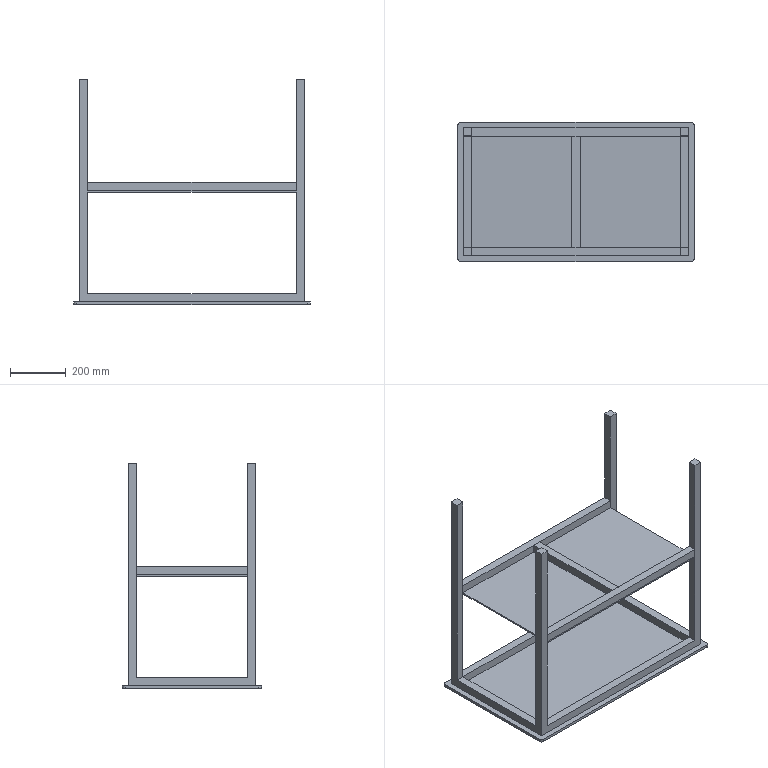Part | SolidWorks | features ICE 6, Extrusion 1, Fillet 1 | 5 solids | 61 faces | box 850 x 500 x 810 mm | volume 12634142 mm3 | plane 57 | cylinder 4 | commonest cylinder face diameters 20 x4